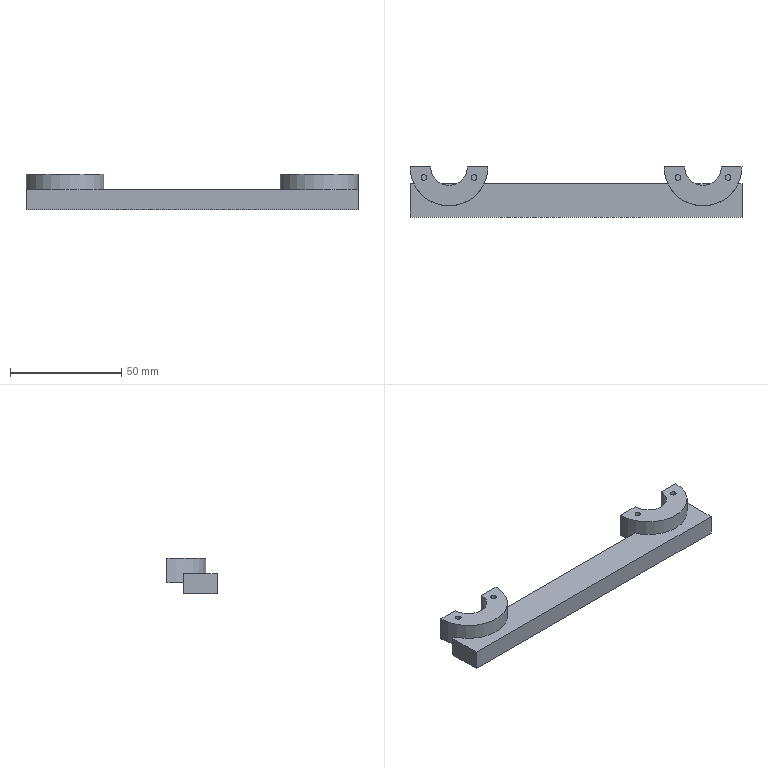NC program | NX | posted with a generic post | part box 149 x 22.5 x 16 mm
Whole program:
N10 G17 G21 G94 G90
(FLOOR_WALL , TOOL : D10)
N12 T02 M6
N14 G54
N16 G17 G0 G90 X52.959 Y-6. S9500 M3
N18 G43 Z30. H2
N20 Z0.025
N22 G94 G1 Z-0.975 F1000.
N24 X56.134 Y-0.5
N26 G2 X57. Y0. R1.
N28 G1 X66.875 F2500.
N30 G3 X47.125 Y0. R12.4
N32 G1 X57.
N34 G2 X57.866 Y-0.5 R1.
N36 G1 X61.041 Y-6.
N38 Z0.025
N40 G0 X52.959 Z-0.95
N42 G1 Z-1.95 F1000.
N44 X56.134 Y-0.5
N46 G2 X57. Y0. R1.
N48 G1 X66.875 F2500.
N50 G3 X47.125 Y0. R12.4
N52 G1 X57.
N54 G2 X57.866 Y-0.5 R1.
N56 G1 X61.041 Y-6.
N58 Z-0.95
N60 G0 X52.959 Z-1.925
N62 G1 Z-2.925 F1000.
N64 X56.134 Y-0.5
N66 G2 X57. Y0. R1.
N68 G1 X66.875 F2500.
N70 G3 X47.125 Y0. R12.4
N72 G1 X57.
N74 G2 X57.866 Y-0.5 R1.
N76 G1 X61.041 Y-6.
N78 Z-1.925
N80 G0 X52.959 Z-2.9
N82 G1 Z-3.9 F1000.
N84 X56.134 Y-0.5
N86 G2 X57. Y0. R1.
N88 G1 X66.875 F2500.
N90 G3 X47.125 Y0. R12.4
N92 G1 X57.
N94 G2 X57.866 Y-0.5 R1.
N96 G1 X61.041 Y-6.
N98 Z-2.9
N100 G0 Z30.
N102 X-61.041
N104 Z0.025
N106 G1 Z-0.975 F1000.
N108 X-57.866 Y-0.5
N110 G2 X-57. Y0. R1.
N112 G1 X-47.125 F2500.
N114 G3 X-66.875 Y0. R12.4
N116 G1 X-57.
N118 G2 X-56.134 Y-0.5 R1.
N120 G1 X-52.959 Y-6.
N122 Z0.025
N124 G0 X-61.041 Z-0.95
N126 G1 Z-1.95 F1000.
N128 X-57.866 Y-0.5
N130 G2 X-57. Y0. R1.
N132 G1 X-47.125 F2500.
N134 G3 X-66.875 Y0. R12.4
N136 G1 X-57.
N138 G2 X-56.134 Y-0.5 R1.
N140 G1 X-52.959 Y-6.
N142 Z-0.95
N144 G0 X-61.041 Z-1.925
N146 G1 Z-2.925 F1000.
N148 X-57.866 Y-0.5
N150 G2 X-57. Y0. R1.
N152 G1 X-47.125 F2500.
N154 G3 X-66.875 Y0. R12.4
N156 G1 X-57.
N158 G2 X-56.134 Y-0.5 R1.
N160 G1 X-52.959 Y-6.
N162 Z-1.925
N164 G0 X-61.041 Z-2.9
N166 G1 Z-3.9 F1000.
N168 X-57.866 Y-0.5
N170 G2 X-57. Y0. R1.
N172 G1 X-47.125 F2500.
N174 G3 X-66.875 Y0. R12.4
N176 G1 X-57.
N178 G2 X-56.134 Y-0.5 R1.
N180 G1 X-52.959 Y-6.
N182 Z-2.9
N184 G0 Z30.
(FLOOR_WALL_COPY , TOOL : D10)
N186 X58.155
N188 Z-3.
N190 G1 Z-4. F1000.
N192 X57.866 Y-5.5
N194 G3 X57. Y-5. R1.
N196 G1 X44.904
N198 X46.158 Y-2.357
N200 G2 X67.842 Y-2.357 R12.
N202 G1 X69.096 Y-5.
N204 X57.
N206 Y-0.5
N208 X54.307
N210 G2 X59.693 Y-0.5 R7.5
N212 G1 X57.
N214 G3 X56.134 Y-1. R1.
N216 G1 Z-3.
N218 G0 X69.566 Y-6.
N220 G1 Z-4.
N222 X69.569 Y-5.997
N224 G3 X69.649 Y-5. R1.
N226 G1 X68.294 Y-2.143
N228 G3 X45.706 Y-2.143 R12.5
N230 G1 X44.351 Y-5.
N232 G3 X44.434 Y-6. R1.
N234 G1 Z-3.
N236 G0 Z30.
N238 X-55.845
N240 Z-3.
N242 G1 Z-4.
N244 X-56.134 Y-5.5
N246 G3 X-57. Y-5. R1.
N248 G1 X-69.096
N250 X-67.842 Y-2.357
N252 G2 X-46.158 Y-2.357 R12.
N254 G1 X-44.904 Y-5.
N256 X-57.
N258 Y-0.5
N260 X-59.693
N262 G2 X-54.307 Y-0.5 R7.5
N264 G1 X-57.
N266 G3 X-57.866 Y-1. R1.
N268 G1 Z-3.
N270 G0 X-44.434 Y-6.
N272 G1 Z-4.
N274 X-44.431 Y-5.997
N276 G3 X-44.351 Y-5. R1.
N278 G1 X-45.706 Y-2.143
N280 G3 X-68.294 Y-2.143 R12.5
N282 G1 X-69.649 Y-5.
N284 G3 X-69.566 Y-6. R1.
N286 G1 Z-3.
N288 G0 Z30.
N290 M5
N292 M2